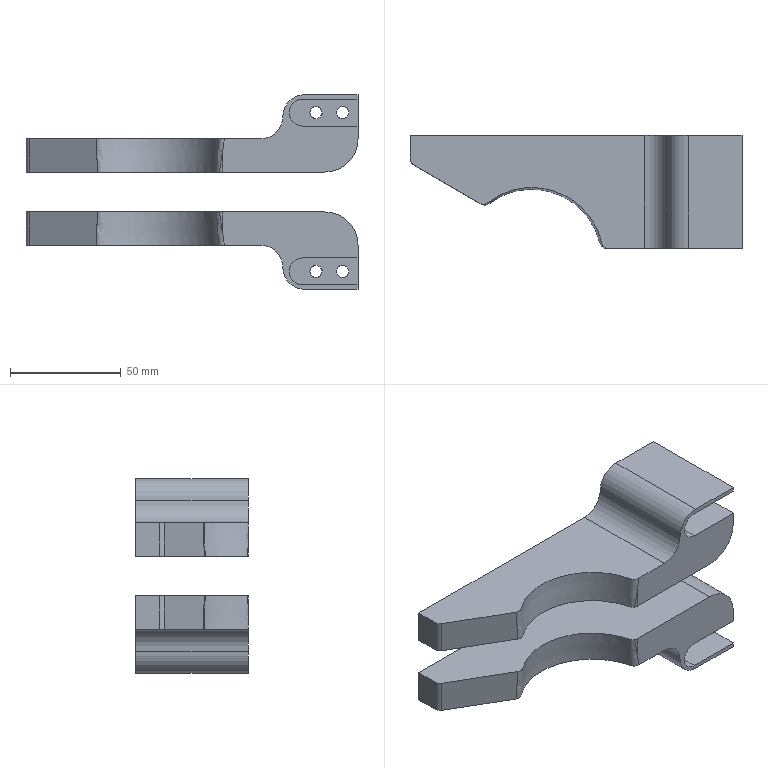NC program | NX | posted with a generic post | part box 150 x 51 x 88 mm
Lines 9164 to 10005 of 21230:
(FIXED_CONTOUR_COPY , TOOL : R4)
N18290 T08 M6
N18292 G54
N18294 G17 G0 G90 X12.055 Y18.193 S9500 M3
N18296 G43 Z30. H8
N18298 Z4.4
N18300 G94 G1 Z0.185 F3000.
N18302 Y18.066 Z0.019
N18304 Y17.9 Z-0.108
N18306 Y17.707 Z-0.188
N18308 Y17.5 Z-0.215
N18310 X12.054 Y13.737 Z-0.213
N18312 X12.065 Y11.855 Z-0.236
N18314 X12.08 Y9.973 Z-0.27
N18316 X12.09 Y9.033 Z-0.29
N18318 X12.106 Y8.383 Z-0.302
N18320 X12.156 Y7.908 Z-0.298
N18322 X12.376 Y6.012 Z-0.279
N18324 X12.618 Y4.124 Z-0.251
N18326 X12.746 Y3.183 Z-0.234
N18328 X12.88 Y2.245 Z-0.219
N18330 X12.781 Y2.244 Z-0.244
N18332 X12.649 Y3.183 Z-0.261
N18334 X12.522 Y4.124 Z-0.279
N18336 X12.28 Y6.011 Z-0.308
N18338 X12.061 Y7.908 Z-0.329
N18340 X12.011 Y8.383 Z-0.333
N18342 X11.995 Y9.033 Z-0.321
N18344 X11.985 Y9.974 Z-0.301
N18346 X11.957 Y13.737 Z-0.239
N18348 X11.958 Y17.5 Z-0.24
N18350 X11.861 Z-0.267
N18352 Y13.737
N18354 X11.89 Y9.974 Z-0.332
N18356 X11.9 Y9.033 Z-0.353
N18358 X11.917 Y8.383 Z-0.365
N18360 X11.967 Y7.907 Z-0.361
N18362 X12.185 Y6.011 Z-0.339
N18364 X12.425 Y4.123 Z-0.308
N18366 X12.552 Y3.182 Z-0.289
N18368 X12.684 Y2.243 Z-0.271
N18370 X12.587 Z-0.299
N18372 X12.456 Y3.182 Z-0.318
N18374 X12.329 Y4.123 Z-0.338
N18376 X12.09 Y6.011 Z-0.371
N18378 X11.873 Y7.907 Z-0.395
N18380 X11.823 Y8.383 Z-0.399
N18382 X11.806 Y9.033 Z-0.387
N18384 X11.796 Y9.974 Z-0.365
N18386 X11.766 Y13.737 Z-0.297
N18388 X11.765 Y17.5 Z-0.295
N18390 X11.669 Z-0.325
N18392 X11.671 Y13.737 Z-0.33
N18394 X11.703 Y9.974 Z-0.399
N18396 X11.713 Y9.033 Z-0.422
N18398 X11.73 Y8.383 Z-0.434
N18400 X11.78 Y7.907 Z-0.429
N18402 X11.996 Y6.011 Z-0.405
N18404 X12.234 Y4.122 Z-0.37
N18406 X12.36 Y3.181 Z-0.349
N18408 X12.491 Y2.242 Z-0.329
N18410 X12.395 Z-0.36
N18412 X12.265 Y3.181 Z-0.381
N18414 X12.14 Y4.122 Z-0.403
N18416 X11.902 Y6.01 Z-0.439
N18418 X11.687 Y7.907 Z-0.465
N18420 X11.638 Y8.383 Z-0.471
N18422 X11.62 Y9.033 Z-0.458
N18424 X11.61 Y9.974 Z-0.435
N18426 X11.578 Y13.737 Z-0.365
N18428 X11.574 Y17.5 Z-0.355
N18430 X11.479 Z-0.387
N18432 X11.485 Y13.737 Z-0.399
N18434 X11.518 Y9.974 Z-0.471
N18436 X11.528 Y9.033 Z-0.495
N18438 X11.546 Y8.383 Z-0.508
N18440 X11.595 Y7.907 Z-0.503
N18442 X11.809 Y6.01 Z-0.475
N18444 X12.046 Y4.122 Z-0.437
N18446 X12.17 Y3.181 Z-0.414
N18448 X12.3 Y2.241 Z-0.392
N18450 X12.205 Z-0.425
N18452 X12.076 Y3.18 Z-0.449
N18454 X11.952 Y4.122 Z-0.473
N18456 X11.717 Y6.01 Z-0.513
N18458 X11.503 Y7.907 Z-0.541
N18460 X11.454 Y8.383 Z-0.547
N18462 X11.437 Y9.033 Z-0.534
N18464 X11.426 Y9.974 Z-0.509
N18466 X11.392 Y13.737 Z-0.435
N18468 X11.386 Y17.5 Z-0.421
N18470 X11.292 Z-0.455
N18472 Y15.618
N18474 X11.3 Y13.737 Z-0.471
N18476 X11.335 Y9.974 Z-0.549
N18478 X11.346 Y9.033 Z-0.574
N18480 X11.364 Y8.383 Z-0.587
N18482 X11.412 Y7.907 Z-0.581
N18484 X11.625 Y6.011 Z-0.551
N18486 X11.859 Y4.122 Z-0.51
N18488 X11.983 Y3.18 Z-0.484
N18490 X12.111 Y2.241 Z-0.46
N18492 X12.017 Z-0.496
N18494 X11.89 Y3.18 Z-0.522
N18496 X11.767 Y4.122 Z-0.548
N18498 X11.534 Y6.011 Z-0.591
N18500 X11.322 Y7.908 Z-0.622
N18502 X11.273 Y8.383 Z-0.629
N18504 X11.256 Y9.033 Z-0.615
N18506 X11.244 Y9.974 Z-0.589
N18508 X11.208 Y13.737 Z-0.51
N18510 X11.199 Y15.618 Z-0.491
N18512 X11.2 Y17.5
N18514 X11.107 Z-0.528
N18516 Y15.618
N18518 X11.117 Y13.737 Z-0.549
N18520 X11.154 Y9.974 Z-0.631
N18522 X11.166 Y9.033 Z-0.657
N18524 X11.184 Y8.383 Z-0.671
N18526 X11.232 Y7.908 Z-0.665
N18528 X11.443 Y6.011 Z-0.632
N18530 X11.676 Y4.122 Z-0.587
N18532 X11.798 Y3.181 Z-0.56
N18534 X11.925 Y2.241 Z-0.533
N18536 X11.832 Z-0.572
N18538 X11.706 Y3.181 Z-0.6
N18540 X11.585 Y4.122 Z-0.628
N18542 X11.353 Y6.011 Z-0.674
N18544 X11.143 Y7.908 Z-0.709
N18546 X11.095 Y8.384 Z-0.715
N18548 X11.077 Y9.033 Z-0.701
N18550 X11.065 Y9.974 Z-0.674
N18552 X11.026 Y13.737 Z-0.59
N18554 X11.016 Y15.618 Z-0.568
N18556 Y17.5 Z-0.567
N18558 X10.925 Z-0.607
N18560 X10.926 Y15.618 Z-0.61
N18562 X10.937 Y13.737 Z-0.632
N18564 X10.976 Y9.974 Z-0.719
N18566 X10.988 Y9.033 Z-0.746
N18568 X11.006 Y8.384 Z-0.761
N18570 X11.054 Y7.909 Z-0.754
N18572 X11.264 Y6.012 Z-0.718
N18574 X11.494 Y4.123 Z-0.67
N18576 X11.615 Y3.181 Z-0.641
N18578 X11.741 Y2.241 Z-0.612
N18580 X11.65 Y2.242 Z-0.653
N18582 X11.525 Y3.181 Z-0.683
N18584 X11.404 Y4.123 Z-0.713
N18586 X11.175 Y6.012 Z-0.763
N18588 X10.966 Y7.909 Z-0.8
N18590 X10.918 Y8.385 Z-0.807
N18592 X10.9 Y9.033 Z-0.792
N18594 X10.888 Y9.974 Z-0.764
N18596 X10.847 Y13.737 Z-0.675
N18598 X10.837 Y15.618 Z-0.652
N18600 X10.835 Y17.5 Z-0.648
N18602 X10.745 Z-0.69
N18604 X10.747 Y15.618 Z-0.695
N18606 X10.758 Y13.737 Z-0.72
N18608 X10.8 Y9.974 Z-0.811
N18610 X10.813 Y9.033 Z-0.84
N18612 X10.831 Y8.385 Z-0.855
N18614 X10.879 Y7.91 Z-0.848
N18616 X11.086 Y6.013 Z-0.809
N18618 X11.315 Y4.124 Z-0.758
N18620 X11.559 Y2.242 Z-0.696
N18622 X11.469 Z-0.74
N18624 X11.226 Y4.124 Z-0.804
N18626 X10.999 Y6.013 Z-0.857
N18628 X10.792 Y7.91 Z-0.896
N18630 X10.744 Y8.386 Z-0.904
N18632 X10.726 Y9.033 Z-0.889
N18634 X10.713 Y9.974 Z-0.859
N18636 X10.67 Y13.737 Z-0.766
N18638 X10.659 Y15.618 Z-0.74
N18640 X10.656 Y17.5 Z-0.734
N18642 X10.567 Z-0.779
N18644 X10.57 Y15.618 Z-0.786
N18646 X10.583 Y13.737 Z-0.813
N18648 X10.626 Y9.974 Z-0.909
N18650 X10.64 Y9.033 Z-0.939
N18652 X10.658 Y8.386 Z-0.955
N18654 X10.706 Y7.911 Z-0.947
N18656 X10.912 Y6.014 Z-0.906
N18658 X11.138 Y4.125 Z-0.851
N18660 X11.38 Y2.243 Z-0.785
N18662 X11.291 Y2.244 Z-0.832
N18664 X11.051 Y4.125 Z-0.9
N18666 X10.825 Y6.015 Z-0.956
N18668 X10.62 Y7.912 Z-0.998
N18670 X10.573 Y8.387 Z-1.006
N18672 X10.554 Y9.033 Z-0.99
N18674 X10.54 Y9.974 Z-0.96
N18676 X10.496 Y13.737 Z-0.861
N18678 X10.483 Y15.618 Z-0.833
N18680 X10.479 Y17.5 Z-0.825
N18682 X10.392 Z-0.872
N18684 X10.396 Y15.618 Z-0.882
N18686 X10.409 Y13.737 Z-0.911
N18688 X10.455 Y9.974 Z-1.012
N18690 X10.469 Y9.033 Z-1.043
N18692 X10.488 Y8.388 Z-1.06
N18694 X10.535 Y7.912 Z-1.051
N18696 X10.739 Y6.016 Z-1.007
N18698 X10.964 Y4.126 Z-0.949
N18700 X11.203 Y2.244 Z-0.879
N18702 X11.116 Y2.245 Z-0.928
N18704 X10.877 Y4.127 Z-1.
N18706 X10.654 Y6.016 Z-1.06
N18708 X10.45 Y7.913 Z-1.105
N18710 X10.404 Y8.389 Z-1.114
N18712 X10.385 Y9.033 Z-1.097
N18714 X10.37 Y9.974 Z-1.065
N18716 X10.323 Y13.737 Z-0.962
N18718 X10.31 Y15.618 Z-0.932
N18720 X10.305 Y17.5 Z-0.921
N18722 X10.218 Z-0.971
N18724 X10.224 Y15.619 Z-0.983
N18726 X10.238 Y13.737 Z-1.015
N18728 X10.286 Y9.974 Z-1.12
N18730 X10.301 Y9.033 Z-1.153
N18732 X10.32 Y8.39 Z-1.17
N18734 X10.367 Y7.914 Z-1.16
N18736 X10.569 Y6.017 Z-1.114
N18738 X10.791 Y4.128 Z-1.053
N18740 X11.029 Y2.246 Z-0.979
N18742 X10.942 Y2.247 Z-1.031
N18744 X10.706 Y4.129 Z-1.107
N18746 X10.485 Y6.018 Z-1.169
N18748 X10.283 Y7.915 Z-1.217
N18750 X10.237 Y8.391 Z-1.227
N18752 X10.218 Y9.033 Z-1.209
N18754 X10.203 Y9.974 Z-1.176
N18756 X10.154 Y13.737 Z-1.068
N18758 X10.139 Y15.619 Z-1.036
N18760 X10.133 Y17.5 Z-1.023
N18762 X10.048 Z-1.075
N18764 X10.054 Y15.619 Z-1.089
N18766 X10.07 Y13.737 Z-1.123
N18768 X10.12 Y9.974 Z-1.234
N18770 X10.135 Y9.033 Z-1.267
N18772 X10.154 Y8.392 Z-1.285
N18774 X10.201 Y7.916 Z-1.275
N18776 X10.401 Y6.02 Z-1.226
N18778 X10.622 Y4.13 Z-1.162
N18780 X10.856 Y2.248 Z-1.084
N18782 X10.771 Y2.249 Z-1.138
N18784 X10.538 Y4.131 Z-1.218
N18786 X10.318 Y6.021 Z-1.284
N18788 X10.119 Y7.917 Z-1.335
N18790 X10.072 Y8.393 Z-1.345
N18792 X10.053 Y9.033 Z-1.327
N18794 X10.038 Y9.974 Z-1.293
N18796 X9.986 Y13.737 Z-1.18
N18798 X9.97 Y15.619 Z-1.145
N18800 X9.963 Y17.5 Z-1.129
N18802 X9.879 Z-1.184
N18804 X9.887 Y15.619 Z-1.201
N18806 X9.903 Y13.737 Z-1.237
N18808 X9.956 Y9.974 Z-1.353
N18810 X9.972 Y9.033 Z-1.388
N18812 X9.991 Y8.394 Z-1.406
N18814 X10.037 Y7.919 Z-1.395
N18816 X10.236 Y6.022 Z-1.344
N18818 X10.454 Y4.133 Z-1.276
N18820 X10.687 Y2.25 Z-1.194
N18822 X10.603 Y2.252 Z-1.251
N18824 X10.372 Y4.134 Z-1.335
N18826 X10.154 Y6.023 Z-1.405
N18828 X9.956 Y7.92 Z-1.458
N18830 X9.91 Y8.395 Z-1.468
N18832 X9.891 Y9.033 Z-1.45
N18834 X9.875 Y9.974 Z-1.414
N18836 X9.821 Y13.737 Z-1.296
N18838 X9.804 Y15.619 Z-1.259
N18840 X9.796 Y17.5 Z-1.241
N18842 X9.713 Z-1.299
N18844 X9.722 Y15.619 Z-1.318
N18846 X9.74 Y13.737 Z-1.357
N18848 X9.794 Y9.974 Z-1.477
N18850 X9.811 Y9.033 Z-1.513
N18852 X9.83 Y8.396 Z-1.532
N18854 X9.876 Y7.921 Z-1.521
N18856 X10.073 Y6.025 Z-1.467
N18858 X10.29 Y4.136 Z-1.396
N18860 X10.519 Y2.253 Z-1.31
N18862 X10.437 Y2.255 Z-1.369
N18864 X10.208 Y4.137 Z-1.458
N18866 X9.993 Y6.026 Z-1.53
N18868 X9.796 Y7.923 Z-1.586
N18870 X9.751 Y8.398 Z-1.597
N18872 X9.731 Y9.033 Z-1.578
N18874 X9.715 Y9.974 Z-1.542
N18876 X9.659 Y13.737 Z-1.418
N18878 X9.64 Y15.619 Z-1.379
N18880 X9.631 Y17.5 Z-1.359
N18882 X9.55 Z-1.419
N18884 X9.56 Y15.619 Z-1.44
N18886 X9.578 Y13.737 Z-1.482
N18888 X9.635 Y9.974 Z-1.607
N18890 X9.653 Y9.034 Z-1.645
N18892 X9.672 Y8.399 Z-1.664
N18894 X9.718 Y7.924 Z-1.653
N18896 X9.913 Y6.028 Z-1.595
N18898 X10.127 Y4.139 Z-1.521
N18900 X10.355 Y2.256 Z-1.431
N18902 X10.273 Y2.258 Z-1.493
N18904 X10.047 Y4.14 Z-1.586
N18906 X9.834 Y6.03 Z-1.662
N18908 X9.639 Y7.926 Z-1.72
N18910 X9.594 Y8.401 Z-1.732
N18912 X9.574 Y9.034 Z-1.713
N18914 X9.557 Y9.974 Z-1.675
N18916 X9.499 Y13.737 Z-1.546
N18918 X9.479 Y15.619 Z-1.504
N18920 X9.469 Y17.5 Z-1.481
N18922 X9.389 Z-1.545
N18924 X9.4 Y15.619 Z-1.568
N18926 X9.42 Y13.737 Z-1.612
N18928 X9.479 Y9.974 Z-1.743
N18930 X9.497 Y9.034 Z-1.782
N18932 X9.517 Y8.402 Z-1.802
N18934 X9.562 Y7.927 Z-1.79
N18936 X9.755 Y6.031 Z-1.73
N18938 X9.967 Y4.142 Z-1.652
N18940 X10.192 Y2.26 Z-1.557
N18942 X10.112 Y2.261 Z-1.623
N18944 X9.889 Y4.144 Z-1.719
N18946 X9.678 Y6.033 Z-1.799
N18948 X9.485 Y7.929 Z-1.86
N18950 X9.44 Y8.404 Z-1.873
N18952 X9.42 Y9.034 Z-1.853
N18954 X9.402 Y9.974 Z-1.813
N18956 X9.341 Y13.737 Z-1.679
N18958 X9.321 Y15.619 Z-1.635
N18960 X9.31 Y17.5 Z-1.61
N18962 X9.231 Z-1.676
N18964 X9.242 Y15.619 Z-1.702
N18966 X9.263 Y13.737 Z-1.748
N18968 X9.326 Y9.974 Z-1.885
N18970 X9.344 Y9.034 Z-1.925
N18972 X9.364 Y8.406 Z-1.945
N18974 X9.409 Y7.931 Z-1.933
N18976 X9.6 Y6.035 Z-1.87
N18978 X9.81 Y4.146 Z-1.788
N18980 X10.033 Y2.263 Z-1.69
N18982 X9.954 Y2.265 Z-1.758
N18984 X9.733 Y4.148 Z-1.859
N18986 X9.524 Y6.037 Z-1.942
N18988 X9.333 Y7.932 Z-2.007
N18990 X9.289 Y8.407 Z-2.02
N18992 X9.268 Y9.034 Z-1.999
N18994 X9.25 Y9.974 Z-1.958
N18996 X9.186 Y13.737 Z-1.819
N18998 X9.165 Y15.619 Z-1.771
N19000 X9.152 Y17.5 Z-1.744
N19002 X9.075 Z-1.813
N19004 X9.088 Y15.619 Z-1.842
N19006 X9.11 Y13.737 Z-1.89
N19008 X9.175 Y9.974 Z-2.033
N19010 X9.194 Y9.034 Z-2.074
N19012 X9.214 Y8.409 Z-2.095
N19014 X9.258 Y7.934 Z-2.082
N19016 X9.448 Y6.039 Z-2.016
N19018 X9.656 Y4.15 Z-1.931
N19020 X9.876 Y2.268 Z-1.828
N19022 X9.798 Y2.27 Z-1.9
N19024 X9.58 Y4.153 Z-2.005
N19026 X9.373 Y6.041 Z-2.092
N19028 X9.184 Y7.936 Z-2.159
N19030 X9.14 Y8.411 Z-2.172
N19032 X9.12 Y9.034 Z-2.151
N19034 X9.1 Y9.974 Z-2.109
N19036 X9.034 Y13.737 Z-1.964
N19038 X9.011 Y15.619 Z-1.914
N19040 X8.998 Y17.5 Z-1.884
N19042 X8.922 Z-1.956
N19044 X8.936 Y15.619 Z-1.987
N19046 X8.959 Y13.737 Z-2.039
N19048 X9.027 Y9.974 Z-2.187
N19050 X9.046 Y9.034 Z-2.23
N19052 X9.067 Y8.413 Z-2.251
N19054 X9.111 Y7.938 Z-2.237
N19056 X9.299 Y6.043 Z-2.169
N19058 X9.504 Y4.155 Z-2.08
N19060 X9.721 Y2.272 Z-1.973
N19062 X9.645 Y2.275 Z-2.047
N19064 X9.429 Y4.157 Z-2.157
N19066 X9.225 Y6.046 Z-2.247
N19068 X9.038 Y7.94 Z-2.318
N19070 X8.994 Y8.415 Z-2.332
N19072 X8.974 Y9.034 Z-2.31
N19074 X8.954 Y9.974 Z-2.266
N19076 X8.885 Y13.737 Z-2.115
N19078 X8.861 Y15.619 Z-2.062
N19080 X8.846 Y17.5 Z-2.03
N19082 X8.772 Z-2.105
N19084 X8.787 Y15.619 Z-2.139
N19086 X8.812 Y13.737 Z-2.193
N19088 X8.882 Y9.975 Z-2.347
N19090 X8.902 Y9.034 Z-2.392
N19092 X8.923 Y8.417 Z-2.414
N19094 X8.966 Y7.943 Z-2.399
N19096 X9.152 Y6.048 Z-2.328
N19098 X9.355 Y4.16 Z-2.235
N19100 X9.57 Y2.277 Z-2.123
N19102 X9.495 Y2.28 Z-2.201
N19104 X9.282 Y4.162 Z-2.315
N19106 X9.08 Y6.051 Z-2.41
N19108 X8.895 Y7.945 Z-2.483
N19110 X8.852 Y8.419 Z-2.498
N19112 X8.831 Y9.034 Z-2.476
N19114 X8.81 Y9.975 Z-2.43
N19116 X8.739 Y13.737 Z-2.273
N19118 X8.713 Y15.619 Z-2.217
N19120 X8.697 Y17.5 Z-2.182
N19122 X8.624 Z-2.261
N19124 X8.641 Y15.619 Z-2.297
N19126 X8.667 Y13.737 Z-2.354
N19128 X8.74 Y9.975 Z-2.515
N19130 X8.761 Y9.034 Z-2.561
N19132 X8.782 Y8.422 Z-2.583
N19134 X8.825 Y7.947 Z-2.568
N19136 X9.009 Y6.053 Z-2.493
N19138 X9.209 Y4.165 Z-2.397
N19140 X9.421 Y2.282 Z-2.28
N19142 X9.348 Y2.285 Z-2.362
N19144 X9.138 Y4.168 Z-2.48
N19146 X8.938 Y6.056 Z-2.579
N19148 X8.755 Y7.95 Z-2.655
N19150 X8.712 Y8.424 Z-2.671
N19152 X8.691 Y9.034 Z-2.648
N19154 X8.67 Y9.975 Z-2.601
N19156 X8.595 Y13.737 Z-2.437
N19158 X8.569 Y15.619 Z-2.378
N19160 X8.552 Y17.5 Z-2.341
N19162 X8.48 Z-2.423
N19164 X8.497 Y15.619 Z-2.462
N19166 X8.525 Y13.737 Z-2.522
N19168 X8.601 Y9.975 Z-2.689
N19170 X8.623 Y9.034 Z-2.737
N19172 X8.644 Y8.426 Z-2.76
N19174 X8.686 Y7.952 Z-2.744
N19176 X8.868 Y6.059 Z-2.666
N19178 X9.067 Y4.171 Z-2.565
N19180 X9.276 Y2.288 Z-2.444
N19182 X9.204 Y2.291 Z-2.529
N19184 X8.996 Y4.174 Z-2.652
N19186 X8.8 Y6.061 Z-2.755
N19188 X8.619 Y7.955 Z-2.835
N19190 X8.576 Y8.429 Z-2.851
N19192 X8.555 Y9.034 Z-2.828
N19194 X8.533 Y9.975 Z-2.779
N19196 X8.455 Y13.737 Z-2.609
N19198 X8.427 Y15.619 Z-2.547
N19200 X8.409 Y17.5 Z-2.506
N19202 X8.338 Z-2.591
N19204 X8.357 Y15.619 Z-2.633
N19206 X8.386 Y13.737 Z-2.697
N19208 X8.465 Y9.975 Z-2.871
N19210 X8.488 Y9.034 Z-2.921
N19212 X8.51 Y8.431 Z-2.944
N19214 X8.552 Y7.957 Z-2.928
N19216 X8.732 Y6.064 Z-2.846
N19218 X8.927 Y4.177 Z-2.741
N19220 X9.133 Y2.294 Z-2.615
N19222 X9.063 Y2.298 Z-2.703
N19224 X8.859 Y4.18 Z-2.832
N19226 X8.664 Y6.068 Z-2.939
N19228 X8.486 Y7.96 Z-3.022
N19230 X8.444 Y8.434 Z-3.039
N19232 X8.422 Y9.034 Z-3.016
N19234 X8.399 Y9.975 Z-2.965
N19236 X8.318 Y13.737 Z-2.787
N19238 X8.289 Y15.619 Z-2.722
N19240 X8.269 Y17.5 Z-2.678
N19242 X8.2 Z-2.767
N19244 X8.221 Y15.619 Z-2.812
N19246 X8.251 Y13.737 Z-2.88
N19248 X8.334 Y9.975 Z-3.061
N19250 X8.357 Y9.034 Z-3.113
N19252 X8.379 Y8.437 Z-3.137
N19254 X8.42 Y7.963 Z-3.119
N19256 X8.598 Y6.071 Z-3.033
N19258 X8.791 Y4.183 Z-2.924
N19260 X8.994 Y2.301 Z-2.793
N19262 X8.926 Y2.304 Z-2.885
N19264 X8.724 Y4.187 Z-3.019
N19266 X8.533 Y6.074 Z-3.13
N19268 X8.356 Y7.966 Z-3.218
N19270 X8.315 Y8.44 Z-3.236
N19272 X8.293 Y9.034 Z-3.212
N19274 X8.269 Y9.975 Z-3.159
N19276 X8.185 Y13.737 Z-2.974
N19278 X8.154 Y15.619 Z-2.905
N19280 X8.133 Y17.5 Z-2.858
N19282 X8.066 Z-2.951
N19284 X8.088 Y15.619 Z-2.999
N19286 X8.12 Y13.737 Z-3.07
N19288 X8.206 Y9.975 Z-3.259
N19290 X8.23 Y9.034 Z-3.313
N19292 X8.252 Y8.443 Z-3.337
N19294 X8.293 Y7.969 Z-3.319
N19296 X8.468 Y6.077 Z-3.229
N19298 X8.658 Y4.19 Z-3.115
N19300 X8.859 Y2.308 Z-2.979
N19302 X8.792 Y2.312 Z-3.075
N19304 X8.594 Y4.194 Z-3.214
N19306 X8.405 Y6.081 Z-3.331
N19308 X8.231 Y7.972 Z-3.422
N19310 X8.19 Y8.446 Z-3.441
N19312 X8.168 Y9.034 Z-3.416
N19314 X8.143 Y9.975 Z-3.361
N19316 X8.055 Y13.737 Z-3.168
N19318 X8.022 Y15.619 Z-3.096
N19320 X8. Y17.5 Z-3.046
N19322 X7.935 Z-3.142
N19324 X7.958 Y15.619 Z-3.194
N19326 X7.992 Y13.737 Z-3.269
N19328 X8.082 Y9.975 Z-3.466
N19330 X8.107 Y9.034 Z-3.522
N19332 X8.129 Y8.449 Z-3.547
N19334 X8.17 Y7.975 Z-3.528
N19336 X8.343 Y6.084 Z-3.434
N19338 X8.53 Y4.198 Z-3.315
N19340 X8.727 Y2.316 Z-3.173
N19342 X8.662 Y2.32 Z-3.273
N19344 X8.467 Y4.202 Z-3.418
N19346 X8.281 Y6.088 Z-3.54
N19348 X8.11 Y7.979 Z-3.636
N19350 X8.07 Y8.452 Z-3.655
N19352 X8.047 Y9.034 Z-3.63
N19354 X8.021 Y9.975 Z-3.573
N19356 X7.93 Y13.737 Z-3.371
N19358 X7.895 Y15.619 Z-3.295
N19360 X7.871 Y17.5 Z-3.241
N19362 X7.807 Z-3.342
N19364 X7.833 Y15.619 Z-3.398
N19366 X7.868 Y13.737 Z-3.476
N19368 X7.962 Y9.975 Z-3.682
N19370 X7.989 Y9.034 Z-3.741
N19372 X8.011 Y8.455 Z-3.766
N19374 X8.051 Y7.982 Z-3.746
N19376 X8.221 Y6.092 Z-3.648
N19378 X8.405 Y4.206 Z-3.524
N19380 X8.599 Y2.324 Z-3.376
N19382 X8.536 Y2.328 Z-3.481
N19384 X8.344 Y4.21 Z-3.632
N19386 X8.162 Y6.096 Z-3.759
N19388 X7.993 Y7.986 Z-3.859
N19390 X7.954 Y8.459 Z-3.88
N19392 X7.931 Y9.034 Z-3.854
N19394 X7.904 Y9.975 Z-3.794
N19396 X7.808 Y13.737 Z-3.584
N19398 X7.771 Y15.619 Z-3.503
N19400 X7.745 Y17.5 Z-3.445
N19402 X7.715 Z-3.498
N19404 X7.684 Z-3.551
N19406 X7.711 Y15.619 Z-3.61
N19408 X7.749 Y13.737 Z-3.693
N19410 X7.847 Y9.975 Z-3.909
N19412 X7.875 Y9.034 Z-3.97
N19414 X7.898 Y8.463 Z-3.996
N19416 X7.937 Y7.99 Z-3.975
N19418 X8.104 Y6.1 Z-3.872
N19420 X8.285 Y4.214 Z-3.742
N19422 X8.475 Y2.332 Z-3.588
N19424 X8.445 Y2.335 Z-3.643
N19426 X8.415 Y2.337 Z-3.698
N19428 X8.227 Y4.219 Z-3.855
N19430 X8.047 Y6.104 Z-3.988
N19432 X7.882 Y7.993 Z-4.094
N19434 X7.843 Y8.466 Z-4.116
N19436 X7.82 Y9.034 Z-4.089
N19438 X7.791 Y9.975 Z-4.027
N19440 X7.691 Y13.737 Z-3.806
N19442 X7.652 Y15.619 Z-3.721
N19444 X7.624 Y17.5 Z-3.659
N19446 X7.595 Z-3.714
N19448 X7.566 Z-3.77
N19450 X7.595 Y15.619 Z-3.833
N19452 X7.634 Y13.737 Z-3.921
N19454 X7.737 Y9.975 Z-4.147
N19456 X7.766 Y9.034 Z-4.211
N19458 X7.789 Y8.47 Z-4.238
N19460 X7.828 Y7.997 Z-4.216
N19462 X7.992 Y6.109 Z-4.107
N19464 X8.169 Y4.223 Z-3.971
N19466 X8.355 Y2.342 Z-3.81
N19468 X8.326 Y2.344 Z-3.867
N19470 X8.298 Y2.346 Z-3.925
N19472 X8.114 Y4.228 Z-4.09
N19474 X7.938 Y6.113 Z-4.229
N19476 X7.775 Y8.002 Z-4.341
N19478 X7.737 Y8.474 Z-4.363
N19480 X7.714 Y9.034 Z-4.336
N19482 X7.684 Y9.975 Z-4.271
N19484 X7.579 Y13.738 Z-4.039
N19486 X7.538 Y15.619 Z-3.949
N19488 X7.521 Y16.559 Z-3.912
N19490 X7.508 Y17.5 Z-3.883
N19492 X7.48 Z-3.94
N19494 X7.452 Z-3.999
N19496 X7.465 Y16.559 Z-4.029
N19498 X7.483 Y15.619 Z-4.067
N19500 X7.525 Y13.738 Z-4.16
N19502 X7.633 Y9.975 Z-4.397
N19504 X7.663 Y9.034 Z-4.464
N19506 X7.687 Y8.478 Z-4.492
N19508 X7.725 Y8.006 Z-4.469
N19510 X7.886 Y6.118 Z-4.355
N19512 X8.059 Y4.233 Z-4.211
N19514 X8.241 Y2.351 Z-4.043
N19516 X8.213 Y2.354 Z-4.103
N19518 X8.186 Y2.357 Z-4.164
N19520 X8.006 Y4.238 Z-4.336
N19522 X7.835 Y6.123 Z-4.483
N19524 X7.675 Y8.01 Z-4.6
N19526 X7.638 Y8.483 Z-4.625
N19528 X7.614 Y9.034 Z-4.597
N19530 X7.583 Y9.975 Z-4.528
N19532 X7.472 Y13.738 Z-4.284
N19534 X7.429 Y15.619 Z-4.188
N19536 X7.411 Y16.559 Z-4.149
N19538 X7.397 Y17.5 Z-4.117
N19540 X7.37 Z-4.178
N19542 X7.343 Z-4.239
N19544 X7.358 Y16.559 Z-4.272
N19546 X7.376 Y15.619 Z-4.313
N19548 X7.421 Y13.738 Z-4.411
N19550 X7.535 Y9.975 Z-4.662
N19552 X7.567 Y9.034 Z-4.732
N19554 X7.591 Y8.487 Z-4.761
N19556 X7.628 Y8.015 Z-4.736
N19558 X7.785 Y6.128 Z-4.615
N19560 X7.954 Y4.244 Z-4.464
N19562 X8.132 Y2.362 Z-4.288
N19564 X8.105 Y2.365 Z-4.351
N19566 X8.079 Y2.368 Z-4.415
N19568 X7.904 Y4.249 Z-4.596
N19570 X7.737 Y6.133 Z-4.751
N19572 X7.582 Y8.02 Z-4.875
N19574 X7.545 Y8.492 Z-4.901
N19576 X7.522 Y9.035 Z-4.872
N19578 X7.489 Y9.975 Z-4.8
N19580 X7.372 Y13.738 Z-4.542
N19582 X7.325 Y15.619 Z-4.44
N19584 X7.306 Y16.559 Z-4.398
N19586 X7.291 Y17.5 Z-4.364
N19588 X7.265 Z-4.428
N19590 X7.24 Z-4.492
N19592 X7.256 Y16.559 Z-4.528
N19594 X7.276 Y15.619 Z-4.571
N19596 X7.324 Y13.738 Z-4.677
N19598 X7.444 Y9.975 Z-4.942
N19600 X7.478 Y9.035 Z-5.017
N19602 X7.502 Y8.496 Z-5.046
N19604 X7.538 Y8.025 Z-5.019
N19606 X7.692 Y6.139 Z-4.891
N19608 X7.856 Y4.255 Z-4.731
N19610 X8.029 Y2.374 Z-4.545
N19612 X8.004 Y2.377 Z-4.612
N19614 X7.979 Y2.38 Z-4.68
N19616 X7.81 Y4.261 Z-4.871
N19618 X7.648 Y6.144 Z-5.035
N19620 X7.497 Y8.03 Z-5.168
N19622 X7.461 Y8.502 Z-5.195
N19624 X7.437 Y9.035 Z-5.166
N19626 X7.402 Y9.975 Z-5.089
N19628 X7.278 Y13.738 Z-4.815
N19630 X7.228 Y15.619 Z-4.706
N19632 X7.208 Y16.559 Z-4.661
N19634 X7.191 Y17.5 Z-4.624
N19636 X7.167 Z-4.692
N19638 X7.144 Z-4.76
N19640 X7.161 Y16.559 Z-4.798
N19642 X7.182 Y15.619 Z-4.845
N19644 X7.234 Y13.738 Z-4.958
N19646 X7.362 Y9.975 Z-5.24
N19648 X7.398 Y9.035 Z-5.32
N19650 X7.422 Y8.507 Z-5.35
N19652 X7.458 Y8.035 Z-5.322
N19654 X7.606 Y6.15 Z-5.184
N19656 X7.765 Y4.267 Z-5.015
N19658 X7.932 Y2.386 Z-4.818
N19660 X7.909 Y2.389 Z-4.889
N19662 X7.887 Y2.392 Z-4.961
N19664 X7.723 Y4.274 Z-5.163
N19666 X7.567 Y6.157 Z-5.339
N19668 X7.42 Y8.041 Z-5.479
N19670 X7.385 Y8.512 Z-5.507
N19672 X7.361 Y9.035 Z-5.477
N19674 X7.324 Y9.975 Z-5.397
N19676 X7.192 Y13.738 Z-5.105
N19678 X7.139 Y15.619 Z-4.989
N19680 X7.116 Y16.559 Z-4.939
N19682 X7.098 Y17.5 Z-4.9
N19684 X7.076 Z-4.971
N19686 X7.055 Z-5.044
N19688 X7.073 Y16.559 Z-5.085
N19690 X7.097 Y15.619 Z-5.137
N19692 X7.152 Y13.738 Z-5.258
N19694 X7.286 Y9.975 Z-5.554
N19696 X7.323 Y9.035 Z-5.634
N19698 X7.347 Y8.517 Z-5.663
N19700 X7.382 Y8.046 Z-5.635
N19702 X7.529 Y6.163 Z-5.496
N19704 X7.683 Y4.28 Z-5.317
N19706 X7.843 Y2.399 Z-5.108
N19708 X7.822 Y2.403 Z-5.183
N19710 X7.802 Y2.406 Z-5.26
N19712 X7.645 Y4.287 Z-5.475
N19714 X7.491 Y6.169 Z-5.654
N19716 X7.343 Y8.052 Z-5.79
N19718 X7.308 Y8.523 Z-5.818
N19720 X7.284 Y9.035 Z-5.789
N19722 X7.248 Y9.975 Z-5.709
N19724 X7.114 Y13.738 Z-5.414
N19726 X7.057 Y15.619 Z-5.29
N19728 X7.033 Y16.559 Z-5.236
N19730 X7.013 Y17.5 Z-5.192
N19732 X6.993 Z-5.269
N19734 X6.974 Z-5.346
N19736 X6.995 Y16.559 Z-5.392
N19738 X7.019 Y15.619 Z-5.446
N19740 X7.076 Y13.738 Z-5.571
N19742 X7.209 Y9.975 Z-5.864
N19744 X7.245 Y9.035 Z-5.943
N19746 X7.268 Y8.528 Z-5.971
N19748 X7.304 Y8.057 Z-5.944
N19750 X7.452 Y6.176 Z-5.81
N19752 X7.607 Y4.294 Z-5.633
N19754 X7.763 Y2.414 Z-5.417
N19756 X7.744 Y2.417 Z-5.497
N19758 X7.725 Y2.421 Z-5.577
N19760 X7.568 Y4.301 Z-5.79
N19762 X7.413 Y6.182 Z-5.964
N19764 X7.264 Y8.063 Z-6.097
N19766 X7.229 Y8.533 Z-6.123
N19768 X7.205 Y9.035 Z-6.095
N19770 X7.17 Y9.975 Z-6.017
N19772 X7.037 Y13.738 Z-5.725
N19774 X6.981 Y15.619 Z-5.602
N19776 X6.957 Y16.559 Z-5.548
N19778 X6.936 Y17.5 Z-5.503
N19780 X6.917 Z-5.581
N19782 X6.898 Z-5.659
N19784 X6.918 Y16.559 Z-5.704
N19786 X6.943 Y15.619 Z-5.757
N19788 X6.998 Y13.738 Z-5.879
N19790 X7.13 Y9.975 Z-6.168
N19792 X7.165 Y9.035 Z-6.247
N19794 X7.188 Y8.538 Z-6.274
N19796 X7.224 Y8.068 Z-6.248
N19798 X7.373 Y6.188 Z-6.118
N19800 X7.529 Y4.308 Z-5.946
N19802 X7.687 Y2.429 Z-5.735
N19804 X7.668 Y2.432 Z-5.814
N19806 X7.648 Y2.436 Z-5.892
N19808 X7.49 Y4.315 Z-6.1
N19810 X7.333 Y6.194 Z-6.27
N19812 X7.183 Y8.073 Z-6.398
N19814 X7.147 Y8.543 Z-6.424
N19816 X7.124 Y9.035 Z-6.397
N19818 X7.089 Y9.975 Z-6.319
N19820 X6.958 Y13.738 Z-6.031
N19822 X6.903 Y15.619 Z-5.91
N19824 X6.879 Y16.559 Z-5.858
N19826 X6.859 Y17.5 Z-5.814
N19828 X6.84 Z-5.891
N19830 X6.82 Z-5.967
N19832 X6.84 Y16.559 Z-6.01
N19834 X6.863 Y15.619 Z-6.062
N19836 X6.918 Y13.738 Z-6.182
N19838 X7.048 Y9.975 Z-6.468
N19840 X7.083 Y9.035 Z-6.546
N19842 X7.106 Y8.548 Z-6.572
N19844 X7.142 Y8.078 Z-6.547
N19846 X7.292 Y6.2 Z-6.42
N19848 X7.449 Y4.322 Z-6.253
N19850 X7.608 Y2.443 Z-6.048
N19852 X7.588 Y2.447 Z-6.125
N19854 X7.568 Y2.45 Z-6.202
N19856 X7.408 Y4.328 Z-6.405
N19858 X7.251 Y6.206 Z-6.57
N19860 X7.1 Y8.083 Z-6.695
N19862 X7.063 Y8.553 Z-6.719
N19864 X7.041 Y9.035 Z-6.693
N19866 X7.006 Y9.975 Z-6.616
N19868 X6.877 Y13.738 Z-6.332
N19870 X6.823 Y15.619 Z-6.213
N19872 X6.8 Y16.559 Z-6.162
N19874 X6.78 Y17.5 Z-6.119
N19876 X6.76 Z-6.195
N19878 X6.74 Z-6.27
N19880 X6.759 Y16.559 Z-6.312
N19882 X6.782 Y15.619 Z-6.363
N19884 X6.835 Y13.738 Z-6.48
N19886 X6.964 Y9.975 Z-6.763
N19888 X6.999 Y9.035 Z-6.84
N19890 X7.021 Y8.557 Z-6.866
N19892 X7.057 Y8.088 Z-6.841
N19894 X7.209 Y6.212 Z-6.719
N19896 X7.367 Y4.335 Z-6.556
N19898 X7.528 Y2.457 Z-6.355
N19900 X7.507 Y2.461 Z-6.431
N19902 X7.486 Y2.464 Z-6.507
N19904 X7.325 Y4.341 Z-6.705
N19906 X7.166 Y6.217 Z-6.866
N19908 X7.014 Y8.093 Z-6.987
N19910 X6.978 Y8.562 Z-7.011
N19912 X6.956 Y9.035 Z-6.986
N19914 X6.921 Y9.975 Z-6.909
N19916 X6.793 Y13.738 Z-6.628
N19918 X6.74 Y15.619 Z-6.511
N19920 X6.717 Y16.559 Z-6.461
N19922 X6.699 Y17.5 Z-6.419
N19924 X6.678 Z-6.494
N19926 X6.657 Z-6.568
N19928 X6.676 Y16.559 Z-6.608
N19930 X6.698 Y15.619 Z-6.658
N19932 X6.751 Y13.738 Z-6.774
N19934 X6.878 Y9.976 Z-7.054
N19936 X6.913 Y9.035 Z-7.13
N19938 X6.934 Y8.567 Z-7.155
N19940 X6.971 Y8.098 Z-7.131
N19942 X7.123 Y6.223 Z-7.012
N19944 X7.283 Y4.347 Z-6.854
N19946 X7.444 Y2.471 Z-6.657
N19948 X7.423 Y2.475 Z-6.732
N19950 X7.402 Y2.478 Z-6.806
N19952 X7.24 Y4.354 Z-7.001
N19954 X7.08 Y6.228 Z-7.157
N19956 X6.927 Y8.103 Z-7.274
N19958 X6.89 Y8.571 Z-7.297
N19960 X6.869 Y9.035 Z-7.273
N19962 X6.834 Y9.976 Z-7.197
N19964 X6.708 Y13.738 Z-6.919
N19966 X6.655 Y15.619 Z-6.804